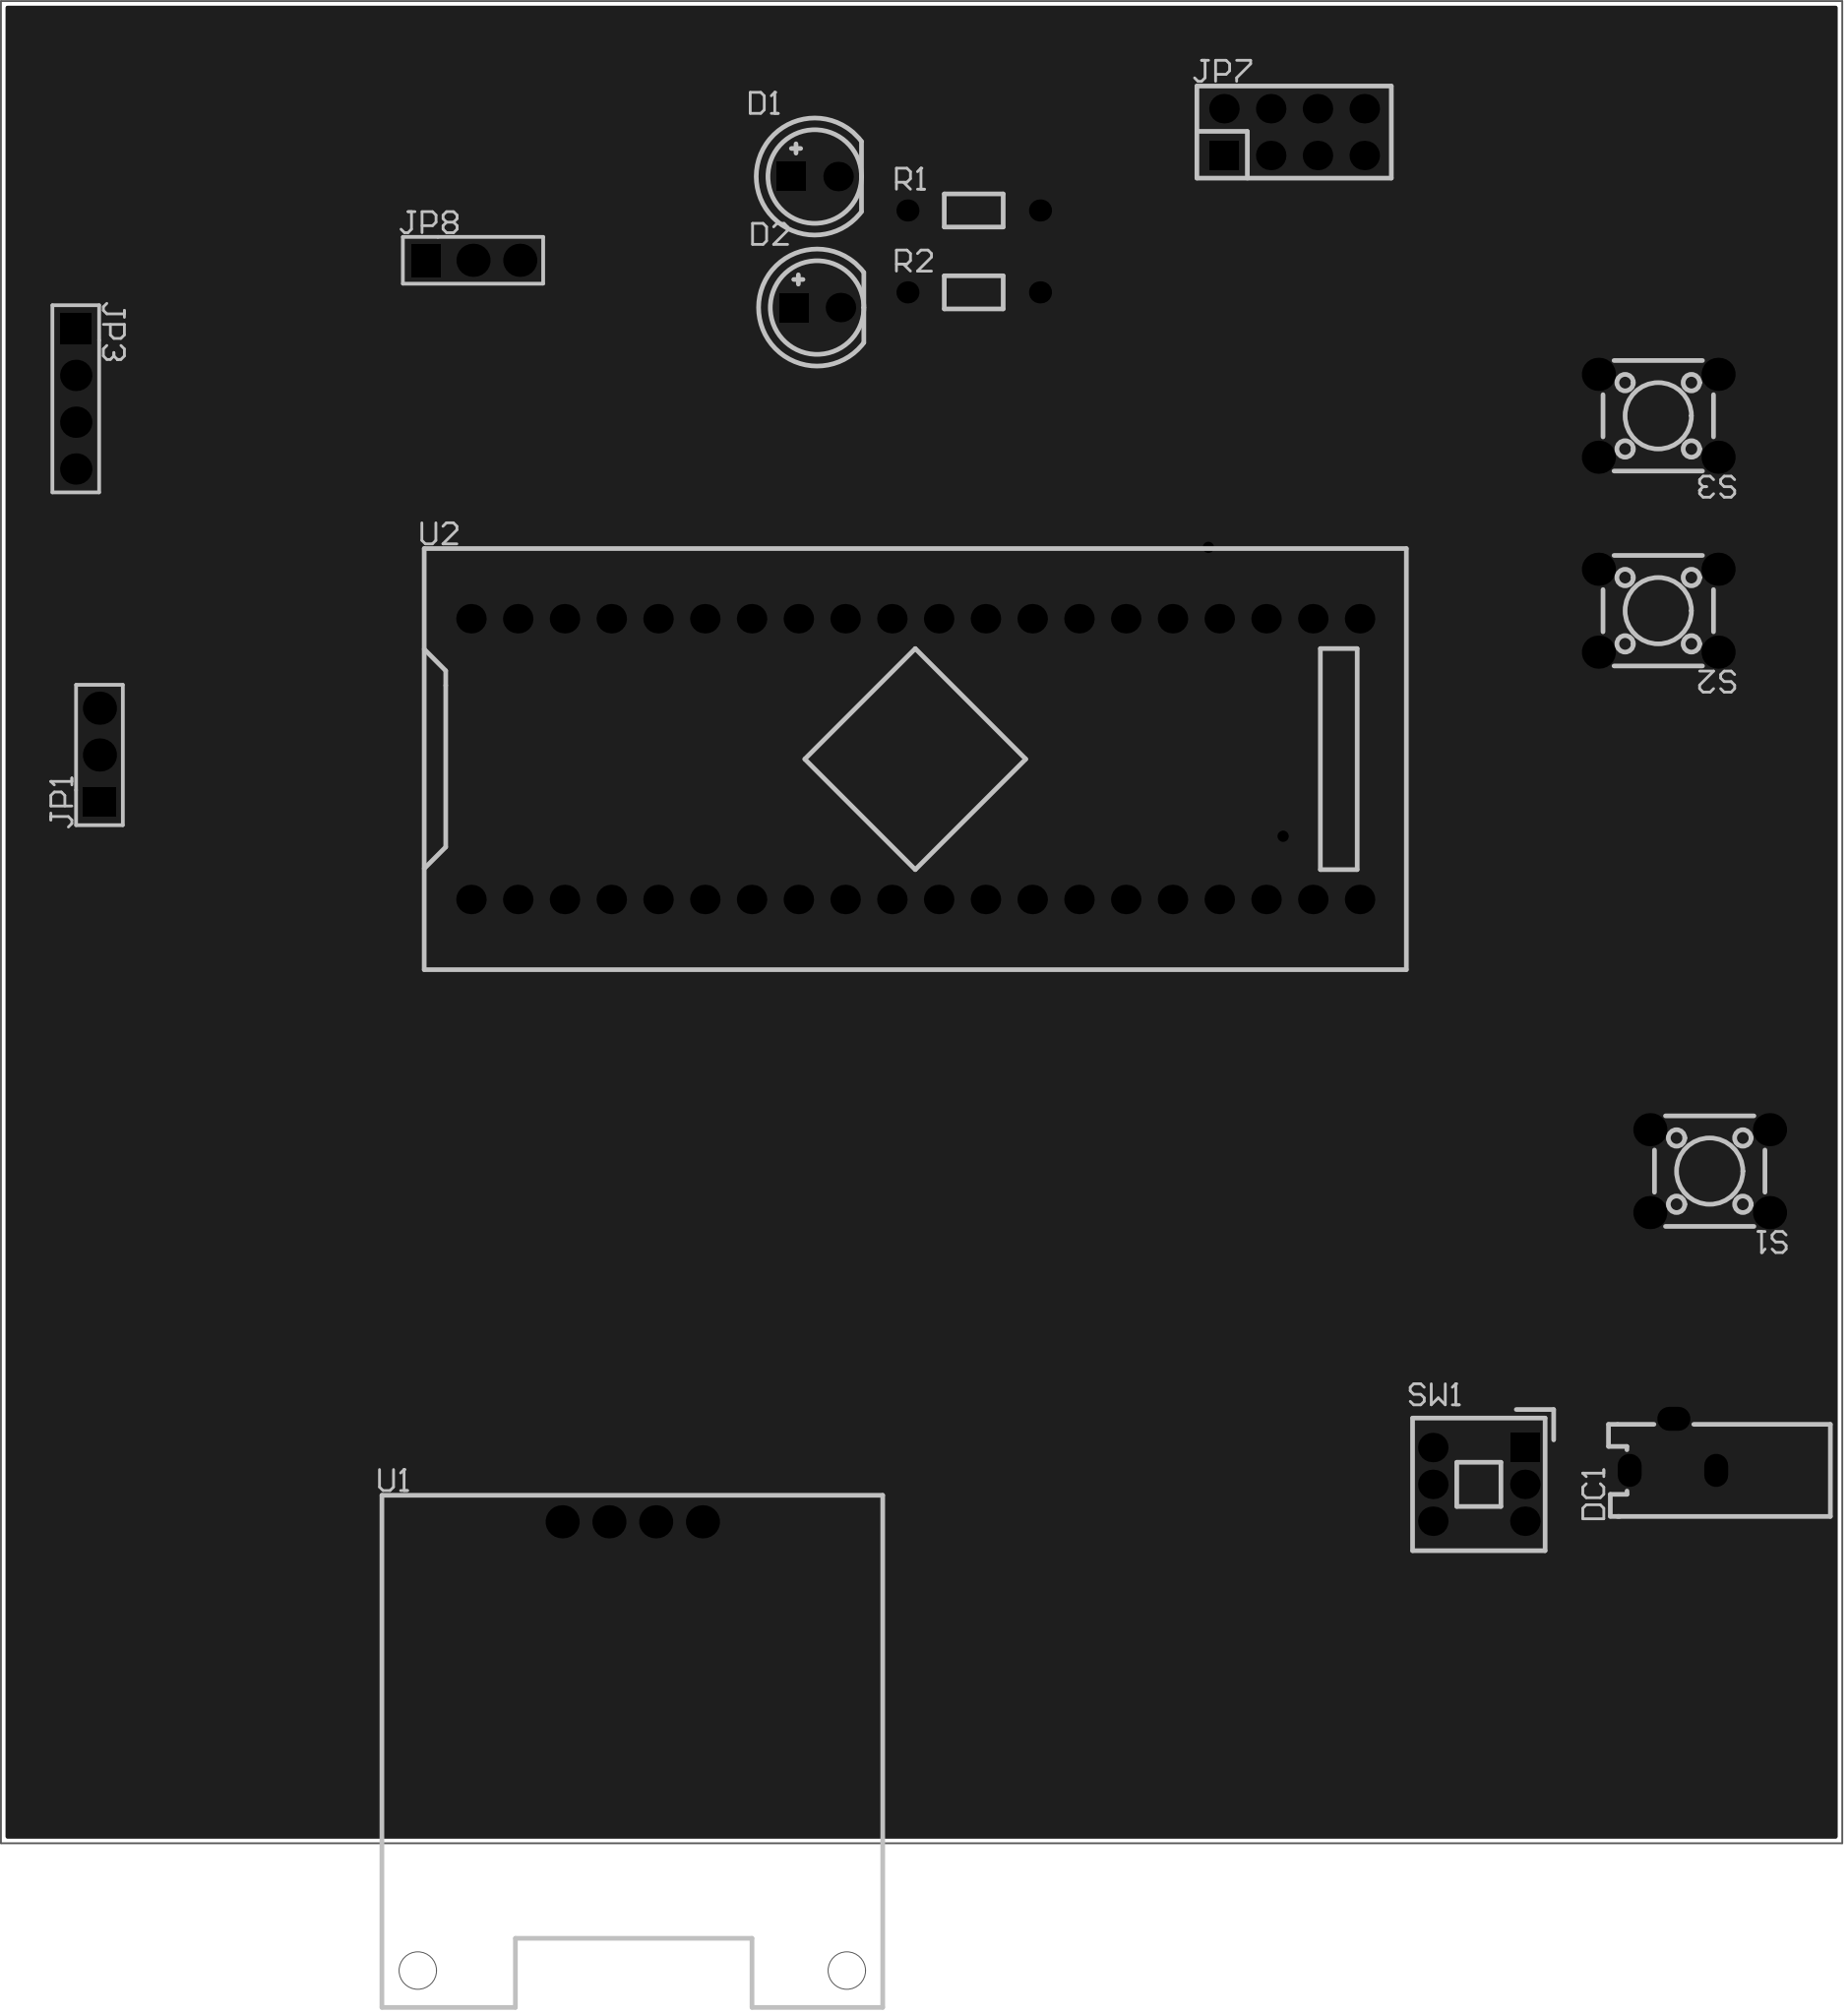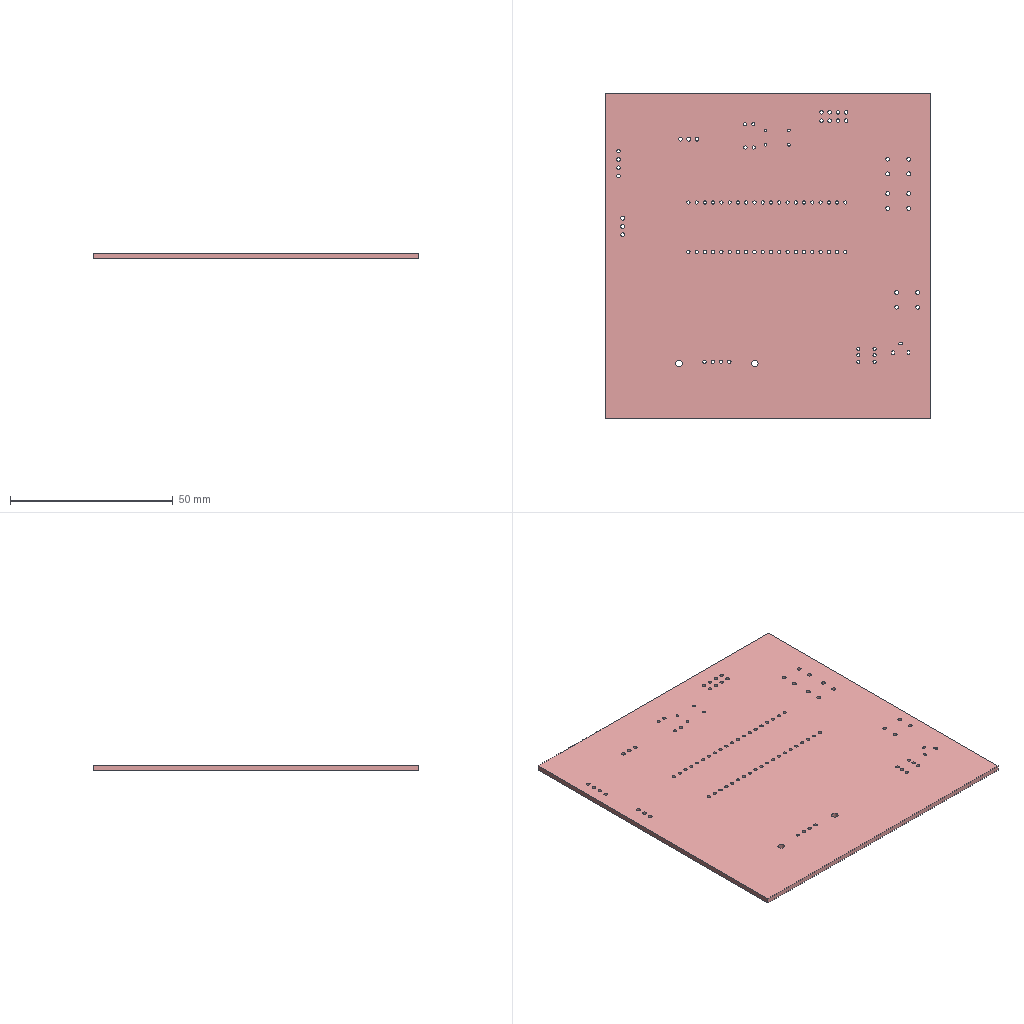Circuit board layout | Altium Designer | box 100 x 100 x 1.6 mm
Layer stack:
# Altium Designer layer stack of  (unit mm; dielectric type: 0 none, 1 core, 2 prepreg, 3 surface material)
index,name,kind,layer,copper_thickness_mm,dielectric_type,dielectric_thickness_mm,dielectric_material,dielectric_constant
0,Top Paste Mask Layer,other,,,,,,
1,Top Silkscreen Layer,other,,,,,,
2,Top Solder Mask Layer,dielectric,,,3,0.01,,3.3
3,Top Layer,copper,Top Layer,0.035,,,,
4,Dielectric1,dielectric,,,3,1.51,FR4,4.5
5,Bottom Layer,copper,Bottom Layer,0.035,,,,
6,Bottom Solder Mask Layer,dielectric,,,3,0.01,,3.3
7,Bottom Silkscreen Layer,other,,,,,,
8,Bottom Paste Mask Layer,other,,,,,,
# drill layer pairs: low layer,high layer
drill_pair,Top Layer,Bottom Layer
Part placement:
Designator,Comment,Layer,Footprint,Center-X(mm),Center-Y(mm),Rotation
D1,led,TopLayer,LED-TH_5mm,129.032,175.712,0
D2,led,TopLayer,LED-TH_5mm,129.159,168.6,0
DC1,DC002-1.3,TopLayer,DC-IN-TH_DC002-1.3,175.641,106.878,90
JP1,HDR-1X3,TopLayer,HDR-TH_3P-P2.54-V-M-1,90.187,144.312,90
JP3,HDR-1X4,TopLayer,HDR-TH_4P-P2.54-V-M-1,88.9,163.647,270
JP7,Header 4X2,TopLayer,HDR-TH_8P-P2.54-V-F-R2-C4-S2.54-1,155.067,178.125,0
JP8,HDR-1X3,TopLayer,HDR-TH_3P-P2.54-V-M-1,110.474,171.165,0
R1,Res2,TopLayer,Res_1/8W,137.668,173.87,0
R2,Res2,TopLayer,Res_1/8W,137.668,169.425,0
S1,key_4,TopLayer,SW-TH_4P-L6.0-W6.0-P4.50-LS6.5,177.637,121.723,180
S2,key_4,TopLayer,SW-TH_4P-L6.0-W6.0-P4.50-LS6.5,174.843,152.144,180
S3,key_4,TopLayer,SW-TH_4P-L6.0-W6.0-P4.50-LS6.5,174.843,162.725,180
SW1,Self-lock button,TopLayer,SW-TH_6P-L7.0-W7.0-P2.00,165.1,104.719,0
U1,OLED,TopLayer,OLED-TH_L27.8-W27.2-P2.54_C9900033791,119.126,102.687,0
U2,STM32F103C8T6-Card,TopLayer,CONN-TH_L53.3-W22.9_STM32F103C8T6-CARD,134.493,144.089,0
Pad and via stacks:
# Altium Designer via and pad stacks of  (unit mm). Each distinct definition once, with the count of objects using it.
# via: kind,start_layer,end_layer,hole_mm,diameter_mm,mode(0 simple;1 top-mid-bottom;2 full stack),diameter_per_layer,count,example_net
# pad: kind,layer,hole_mm,hole_type(0 round;1 square;2 slot),plating,top_size,top_shape(1 round;2 rect;3 octagon;9 rounded rect),mid_size,bottom_size,mode,footprint,size_per_layer,count,example
pad,Multi-Layer,1,0,plated,1.6x1.6,2,1.6x1.6,1.6x1.6,0,LED-TH_5mm,,2,D1.1
pad,Multi-Layer,1,0,plated,1.6x1.6,1,1.6x1.6,1.6x1.6,0,LED-TH_5mm,,2,D1.2
pad,Multi-Layer,0.8,2,plated,1.3x1.8,1,1.3x1.8,1.3x1.8,0,DC-IN-TH_DC002-1.3,,3,DC1.1
pad,Multi-Layer,1.2,0,plated,1.8x1.8,1,1.8x1.8,1.8x1.8,0,HDR-TH_3P-P2.54-V-M-1,,4,JP1.3
pad,Multi-Layer,1.2,0,plated,1.575x1.8,2,1.575x1.8,1.575x1.8,0,HDR-TH_3P-P2.54-V-M-1,,2,JP1.1
pad,Multi-Layer,1.1,0,plated,1.7x1.7,2,1.7x1.7,1.7x1.7,0,HDR-TH_4P-P2.54-V-M-1,,1,JP3.1
pad,Multi-Layer,1.1,0,plated,1.7x1.7,1,1.7x1.7,1.7x1.7,0,HDR-TH_4P-P2.54-V-M-1,,3,JP3.2
pad,Multi-Layer,1.1,0,plated,1.6x1.6,2,1.6x1.6,1.6x1.6,0,HDR-TH_8P-P2.54-V-F-R2-C4-S2.54-1,,1,JP7.1
pad,Multi-Layer,1.1,0,plated,1.6x1.6,1,1.6x1.6,1.6x1.6,0,HDR-TH_8P-P2.54-V-F-R2-C4-S2.54-1,,7,JP7.2
pad,Multi-Layer,0.8001,0,plated,1.199x1.199,1,1.199x1.199,1.199x1.199,0,Res_1/8W,,4,R1.1
pad,Multi-Layer,1.2,0,plated,1.8x1.8,1,1.8x1.8,1.8x1.8,0,SW-TH_4P-L6.0-W6.0-P4.50-LS6.5,,12,S1.1
pad,Multi-Layer,1,0,plated,1.6x1.6,1,1.6x1.6,1.6x1.6,0,SW-TH_6P-L7.0-W7.0-P2.00,,5,SW1.4
pad,Multi-Layer,1,0,plated,1.6x1.6,2,1.6x1.6,1.6x1.6,0,SW-TH_6P-L7.0-W7.0-P2.00,,1,SW1.1
pad,Multi-Layer,1.05,0,plated,1.8x1.8,1,1.8x1.8,1.8x1.8,0,OLED-TH_L27.8-W27.2-P2.54_C9900033791,,4,U1.1
pad,Multi-Layer,1,0,plated,1.6x1.6,1,1.6x1.6,1.6x1.6,0,CONN-TH_L53.3-W22.9_STM32F103C8T6-CARD,,40,U2.1
via,Top Layer,Bottom Layer,0.3048,0.61,0,,2,PB9
Copper pours:
name,layer,net,type(0 solid;1 hatched;2 none)
Top Layer-GND,Top Layer,GND,0
Bottom Layer-GND,Bottom Layer,GND,0
Design rules, without the lines most boards share:
# Altium Designer design rules of  (exported by Altium Designer, unit mm)
# columns: name | kind | enabled | priority | scope1 | scope2 | descriptor | typed fields (field=value)
creepage | 65 | enabled | 1 | All | All | Creepage Distance Constraint =(0mil) (All),(All) |
copperThickness1oz_2 | 2 | enabled | 2 | All | All | Width Constraint (Min=30mil) (Max=100mil) (Preferred=30mil) (All) |